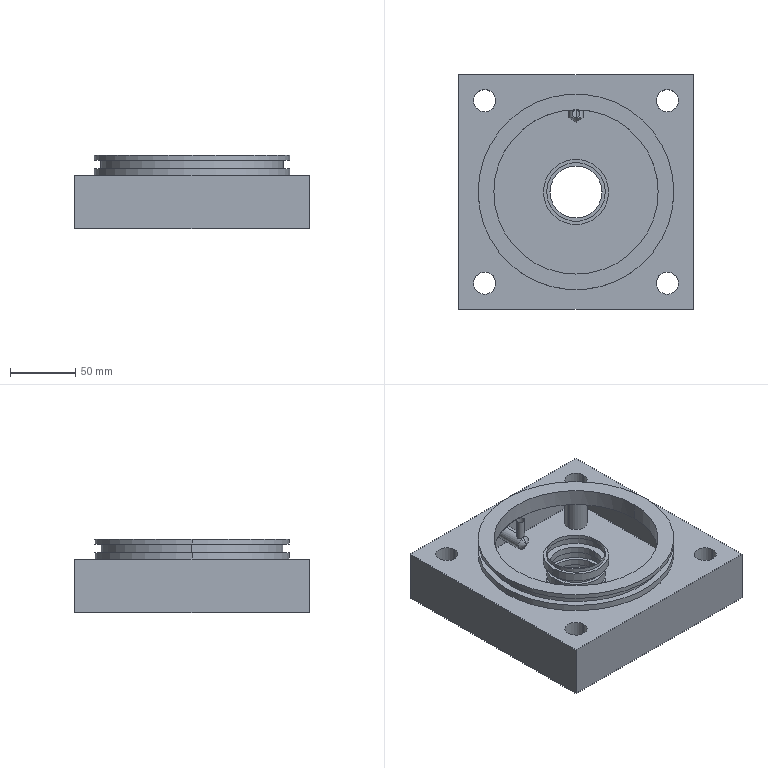Part | SolidWorks | features ICE 4, RevCut 2, Extrusion 1, HoleWzd 1 | 1 solid | 61 faces | box 180 x 180 x 56 mm | volume 1310949 mm3 | cylinder 38 | plane 19 | cone 4 | commonest cylinder face diameters 17 x8 40 x8 45 x8 150 x4 6 x2 11.125 x2